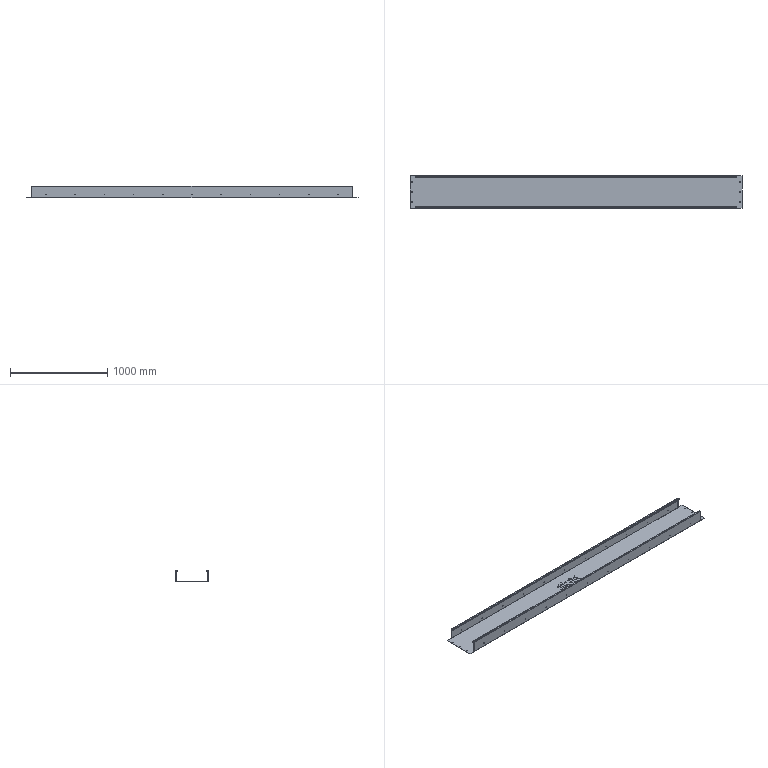Part | STEP file | TS-S25 TBD | 1 solid | 278 faces | box 3411 x 330 x 120 mm | volume 4130819 mm3 | plane 133 | cylinder 112 | spline 33 | commonest cylinder face diameters 5.4 x88 7 x12 0.4 x6 4.4 x6